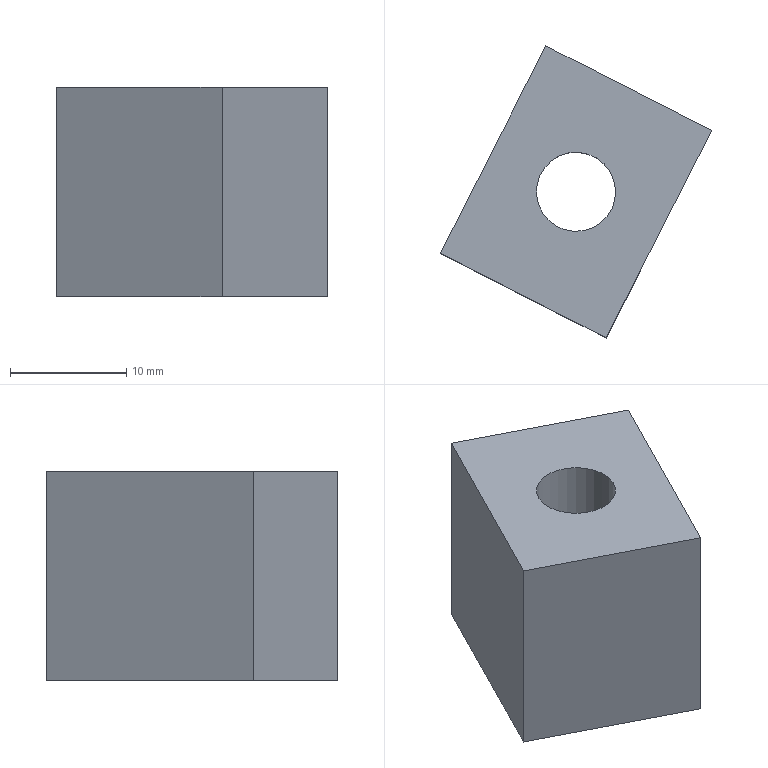Part | STEP file | gslz 2016.10.28-13_id1826_x_t | 1 solid | 9 faces | box 23.336 x 25.084 x 18 mm | volume 4338 mm3 | plane 7 | cylinder 2 | commonest cylinder face diameters 6.8 x1 12 x1
STEP:
#1=CARTESIAN_POINT('',(0.,0.,0.));
#2=DIRECTION('',(0.,0.,1.));
#3=DIRECTION('',(1.,0.,0.));
#4=AXIS2_PLACEMENT_3D('',#1,#2,#3);
#5=CARTESIAN_POINT('',(1096.964,-63.507,-70.5));
#6=VERTEX_POINT('',#5);
#7=CARTESIAN_POINT('',(1106.043,-45.687,-70.5));
#8=VERTEX_POINT('',#7);
#9=CARTESIAN_POINT('',(1103.234,-51.201,-70.5));
#10=DIRECTION('',(0.454,0.891,0.));
#11=VECTOR('',#10,1.);
#12=LINE('',#9,#11);
#13=CARTESIAN_POINT('',(1096.056,-65.289,-97.82));
#14=DIRECTION('',(-0.891,0.454,0.));
#15=DIRECTION('',(0.454,0.891,0.));
#16=AXIS2_PLACEMENT_3D('',#13,#14,#15);
#17=PLANE('',#16);
#18=CARTESIAN_POINT('',(15.812,-27.32));
#19=DIRECTION('',(1.,0.));
#20=VECTOR('',#19,1.);
#21=LINE('',#18,#20);
#22=(GEOMETRIC_REPRESENTATION_CONTEXT(2)PARAMETRIC_REPRESENTATION_CONTEXT()REPRESENTATION_CONTEXT('',''));
#23=DEFINITIONAL_REPRESENTATION('',(#21),#22);
#24=PCURVE('',#17,#23);
#25=CARTESIAN_POINT('',(1099.199,-49.145,-70.5));
#26=DIRECTION('',(0.,0.,1.));
#27=DIRECTION('',(-0.309,0.9511,0.));
#28=AXIS2_PLACEMENT_3D('',#25,#26,#27);
#29=PLANE('',#28);
#30=CARTESIAN_POINT('',(-3.202,-3.202));
#31=DIRECTION('',(0.7071,-0.7071));
#32=VECTOR('',#31,1.);
#33=LINE('',#30,#32);
#34=(GEOMETRIC_REPRESENTATION_CONTEXT(2)PARAMETRIC_REPRESENTATION_CONTEXT()REPRESENTATION_CONTEXT('',''));
#35=DEFINITIONAL_REPRESENTATION('',(#33),#34);
#36=PCURVE('',#29,#35);
#37=SURFACE_CURVE('',#12,(#24,#36),.PCURVE_S1.);
#38=EDGE_CURVE('',#6,#8,#37,.T.);
#39=ORIENTED_EDGE('',*,*,#38,.T.);
#40=CARTESIAN_POINT('',(1106.043,-45.687,-88.5));
#41=VERTEX_POINT('',#40);
#42=CARTESIAN_POINT('',(1106.043,-45.687,-97.82));
#43=DIRECTION('',(0.,0.,1.));
#44=VECTOR('',#43,1.);
#45=LINE('',#42,#44);
#46=CARTESIAN_POINT('',(22.,0.));
#47=DIRECTION('',(0.,-1.));
#48=VECTOR('',#47,1.);
#49=LINE('',#46,#48);
#50=(GEOMETRIC_REPRESENTATION_CONTEXT(2)PARAMETRIC_REPRESENTATION_CONTEXT()REPRESENTATION_CONTEXT('',''));
#51=DEFINITIONAL_REPRESENTATION('',(#49),#50);
#52=PCURVE('',#17,#51);
#53=CARTESIAN_POINT('',(1102.479,-43.871,-97.82));
#54=DIRECTION('',(0.454,0.891,0.));
#55=DIRECTION('',(0.891,-0.454,0.));
#56=AXIS2_PLACEMENT_3D('',#53,#54,#55);
#57=PLANE('',#56);
#58=CARTESIAN_POINT('',(4.,0.));
#59=DIRECTION('',(0.,-1.));
#60=VECTOR('',#59,1.);
#61=LINE('',#58,#60);
#62=(GEOMETRIC_REPRESENTATION_CONTEXT(2)PARAMETRIC_REPRESENTATION_CONTEXT()REPRESENTATION_CONTEXT('',''));
#63=DEFINITIONAL_REPRESENTATION('',(#61),#62);
#64=PCURVE('',#57,#63);
#65=SURFACE_CURVE('',#45,(#52,#64),.PCURVE_S1.);
#66=EDGE_CURVE('',#41,#8,#65,.T.);
#67=ORIENTED_EDGE('',*,*,#66,.F.);
#68=CARTESIAN_POINT('',(1096.964,-63.507,-88.5));
#69=VERTEX_POINT('',#68);
#70=CARTESIAN_POINT('',(1103.234,-51.201,-88.5));
#71=DIRECTION('',(0.454,0.891,0.));
#72=VECTOR('',#71,1.);
#73=LINE('',#70,#72);
#74=CARTESIAN_POINT('',(15.812,-9.32));
#75=DIRECTION('',(1.,0.));
#76=VECTOR('',#75,1.);
#77=LINE('',#74,#76);
#78=(GEOMETRIC_REPRESENTATION_CONTEXT(2)PARAMETRIC_REPRESENTATION_CONTEXT()REPRESENTATION_CONTEXT('',''));
#79=DEFINITIONAL_REPRESENTATION('',(#77),#78);
#80=PCURVE('',#17,#79);
#81=CARTESIAN_POINT('',(1099.199,-49.145,-88.5));
#82=DIRECTION('',(0.,0.,1.));
#83=DIRECTION('',(-0.309,0.9511,0.));
#84=AXIS2_PLACEMENT_3D('',#81,#82,#83);
#85=PLANE('',#84);
#86=CARTESIAN_POINT('',(-3.202,-3.202));
#87=DIRECTION('',(0.7071,-0.7071));
#88=VECTOR('',#87,1.);
#89=LINE('',#86,#88);
#90=(GEOMETRIC_REPRESENTATION_CONTEXT(2)PARAMETRIC_REPRESENTATION_CONTEXT()REPRESENTATION_CONTEXT('',''));
#91=DEFINITIONAL_REPRESENTATION('',(#89),#90);
#92=PCURVE('',#85,#91);
#93=SURFACE_CURVE('',#73,(#80,#92),.PCURVE_S1.);
#94=EDGE_CURVE('',#69,#41,#93,.T.);
#95=ORIENTED_EDGE('',*,*,#94,.F.);
#96=CARTESIAN_POINT('',(1096.964,-63.507,-97.82));
#97=DIRECTION('',(0.,0.,1.));
#98=VECTOR('',#97,1.);
#99=LINE('',#96,#98);
#100=CARTESIAN_POINT('',(2.,0.));
#101=DIRECTION('',(0.,-1.));
#102=VECTOR('',#101,1.);
#103=LINE('',#100,#102);
#104=(GEOMETRIC_REPRESENTATION_CONTEXT(2)PARAMETRIC_REPRESENTATION_CONTEXT()REPRESENTATION_CONTEXT('',''));
#105=DEFINITIONAL_REPRESENTATION('',(#103),#104);
#106=PCURVE('',#17,#105);
#107=CARTESIAN_POINT('',(1114.784,-72.587,-97.82));
#108=DIRECTION('',(-0.454,-0.891,0.));
#109=DIRECTION('',(-0.891,0.454,0.));
#110=AXIS2_PLACEMENT_3D('',#107,#108,#109);
#111=PLANE('',#110);
#112=CARTESIAN_POINT('',(20.,0.));
#113=DIRECTION('',(0.,-1.));
#114=VECTOR('',#113,1.);
#115=LINE('',#112,#114);
#116=(GEOMETRIC_REPRESENTATION_CONTEXT(2)PARAMETRIC_REPRESENTATION_CONTEXT()REPRESENTATION_CONTEXT('',''));
#117=DEFINITIONAL_REPRESENTATION('',(#115),#116);
#118=PCURVE('',#111,#117);
#119=SURFACE_CURVE('',#99,(#106,#118),.PCURVE_S1.);
#120=EDGE_CURVE('',#69,#6,#119,.T.);
#121=ORIENTED_EDGE('',*,*,#120,.T.);
#122=EDGE_LOOP('',(#39,#67,#95,#121));
#123=FACE_BOUND('',#122,.T.);
#124=ADVANCED_FACE('',(#123),#17,.T.);
#125=CARTESIAN_POINT('',(1120.299,-52.951,-70.5));
#126=VERTEX_POINT('',#125);
#127=CARTESIAN_POINT('',(1102.008,-43.631,-70.5));
#128=DIRECTION('',(0.891,-0.454,0.));
#129=VECTOR('',#128,1.);
#130=LINE('',#127,#129);
#131=CARTESIAN_POINT('',(-0.5289,-27.32));
#132=DIRECTION('',(1.,0.));
#133=VECTOR('',#132,1.);
#134=LINE('',#131,#133);
#135=(GEOMETRIC_REPRESENTATION_CONTEXT(2)PARAMETRIC_REPRESENTATION_CONTEXT()REPRESENTATION_CONTEXT('',''));
#136=DEFINITIONAL_REPRESENTATION('',(#134),#135);
#137=PCURVE('',#57,#136);
#138=CARTESIAN_POINT('',(4.376,-4.376));
#139=DIRECTION('',(-0.7071,-0.7071));
#140=VECTOR('',#139,1.);
#141=LINE('',#138,#140);
#142=(GEOMETRIC_REPRESENTATION_CONTEXT(2)PARAMETRIC_REPRESENTATION_CONTEXT()REPRESENTATION_CONTEXT('',''));
#143=DEFINITIONAL_REPRESENTATION('',(#141),#142);
#144=PCURVE('',#29,#143);
#145=SURFACE_CURVE('',#130,(#137,#144),.PCURVE_S1.);
#146=EDGE_CURVE('',#8,#126,#145,.T.);
#147=ORIENTED_EDGE('',*,*,#146,.T.);
#148=CARTESIAN_POINT('',(1120.299,-52.951,-88.5));
#149=VERTEX_POINT('',#148);
#150=CARTESIAN_POINT('',(1120.299,-52.951,-97.82));
#151=DIRECTION('',(0.,0.,1.));
#152=VECTOR('',#151,1.);
#153=LINE('',#150,#152);
#154=CARTESIAN_POINT('',(20.,0.));
#155=DIRECTION('',(0.,-1.));
#156=VECTOR('',#155,1.);
#157=LINE('',#154,#156);
#158=(GEOMETRIC_REPRESENTATION_CONTEXT(2)PARAMETRIC_REPRESENTATION_CONTEXT()REPRESENTATION_CONTEXT('',''));
#159=DEFINITIONAL_REPRESENTATION('',(#157),#158);
#160=PCURVE('',#57,#159);
#161=CARTESIAN_POINT('',(1121.207,-51.169,-97.82));
#162=DIRECTION('',(0.891,-0.454,0.));
#163=DIRECTION('',(-0.454,-0.891,0.));
#164=AXIS2_PLACEMENT_3D('',#161,#162,#163);
#165=PLANE('',#164);
#166=CARTESIAN_POINT('',(2.,0.));
#167=DIRECTION('',(0.,-1.));
#168=VECTOR('',#167,1.);
#169=LINE('',#166,#168);
#170=(GEOMETRIC_REPRESENTATION_CONTEXT(2)PARAMETRIC_REPRESENTATION_CONTEXT()REPRESENTATION_CONTEXT('',''));
#171=DEFINITIONAL_REPRESENTATION('',(#169),#170);
#172=PCURVE('',#165,#171);
#173=SURFACE_CURVE('',#153,(#160,#172),.PCURVE_S1.);
#174=EDGE_CURVE('',#149,#126,#173,.T.);
#175=ORIENTED_EDGE('',*,*,#174,.F.);
#176=CARTESIAN_POINT('',(1102.008,-43.631,-88.5));
#177=DIRECTION('',(0.891,-0.454,0.));
#178=VECTOR('',#177,1.);
#179=LINE('',#176,#178);
#180=CARTESIAN_POINT('',(-0.5289,-9.32));
#181=DIRECTION('',(1.,0.));
#182=VECTOR('',#181,1.);
#183=LINE('',#180,#182);
#184=(GEOMETRIC_REPRESENTATION_CONTEXT(2)PARAMETRIC_REPRESENTATION_CONTEXT()REPRESENTATION_CONTEXT('',''));
#185=DEFINITIONAL_REPRESENTATION('',(#183),#184);
#186=PCURVE('',#57,#185);
#187=CARTESIAN_POINT('',(4.376,-4.376));
#188=DIRECTION('',(-0.7071,-0.7071));
#189=VECTOR('',#188,1.);
#190=LINE('',#187,#189);
#191=(GEOMETRIC_REPRESENTATION_CONTEXT(2)PARAMETRIC_REPRESENTATION_CONTEXT()REPRESENTATION_CONTEXT('',''));
#192=DEFINITIONAL_REPRESENTATION('',(#190),#191);
#193=PCURVE('',#85,#192);
#194=SURFACE_CURVE('',#179,(#186,#193),.PCURVE_S1.);
#195=EDGE_CURVE('',#41,#149,#194,.T.);
#196=ORIENTED_EDGE('',*,*,#195,.F.);
#197=ORIENTED_EDGE('',*,*,#66,.T.);
#198=EDGE_LOOP('',(#147,#175,#196,#197));
#199=FACE_BOUND('',#198,.T.);
#200=ADVANCED_FACE('',(#199),#57,.T.);
#201=CARTESIAN_POINT('',(1111.22,-70.771,-70.5));
#202=VERTEX_POINT('',#201);
#203=CARTESIAN_POINT('',(1117.49,-58.465,-70.5));
#204=DIRECTION('',(-0.454,-0.891,0.));
#205=VECTOR('',#204,1.);
#206=LINE('',#203,#205);
#207=CARTESIAN_POINT('',(8.188,-27.32));
#208=DIRECTION('',(1.,0.));
#209=VECTOR('',#208,1.);
#210=LINE('',#207,#209);
#211=(GEOMETRIC_REPRESENTATION_CONTEXT(2)PARAMETRIC_REPRESENTATION_CONTEXT()REPRESENTATION_CONTEXT('',''));
#212=DEFINITIONAL_REPRESENTATION('',(#210),#211);
#213=PCURVE('',#165,#212);
#214=CARTESIAN_POINT('',(-14.516,-14.516));
#215=DIRECTION('',(-0.7071,0.7071));
#216=VECTOR('',#215,1.);
#217=LINE('',#214,#216);
#218=(GEOMETRIC_REPRESENTATION_CONTEXT(2)PARAMETRIC_REPRESENTATION_CONTEXT()REPRESENTATION_CONTEXT('',''));
#219=DEFINITIONAL_REPRESENTATION('',(#217),#218);
#220=PCURVE('',#29,#219);
#221=SURFACE_CURVE('',#206,(#213,#220),.PCURVE_S1.);
#222=EDGE_CURVE('',#126,#202,#221,.T.);
#223=ORIENTED_EDGE('',*,*,#222,.T.);
#224=CARTESIAN_POINT('',(1111.22,-70.771,-88.5));
#225=VERTEX_POINT('',#224);
#226=CARTESIAN_POINT('',(1111.22,-70.771,-97.82));
#227=DIRECTION('',(0.,0.,1.));
#228=VECTOR('',#227,1.);
#229=LINE('',#226,#228);
#230=CARTESIAN_POINT('',(22.,0.));
#231=DIRECTION('',(0.,-1.));
#232=VECTOR('',#231,1.);
#233=LINE('',#230,#232);
#234=(GEOMETRIC_REPRESENTATION_CONTEXT(2)PARAMETRIC_REPRESENTATION_CONTEXT()REPRESENTATION_CONTEXT('',''));
#235=DEFINITIONAL_REPRESENTATION('',(#233),#234);
#236=PCURVE('',#165,#235);
#237=CARTESIAN_POINT('',(4.,0.));
#238=DIRECTION('',(0.,-1.));
#239=VECTOR('',#238,1.);
#240=LINE('',#237,#239);
#241=(GEOMETRIC_REPRESENTATION_CONTEXT(2)PARAMETRIC_REPRESENTATION_CONTEXT()REPRESENTATION_CONTEXT('',''));
#242=DEFINITIONAL_REPRESENTATION('',(#240),#241);
#243=PCURVE('',#111,#242);
#244=SURFACE_CURVE('',#229,(#236,#243),.PCURVE_S1.);
#245=EDGE_CURVE('',#225,#202,#244,.T.);
#246=ORIENTED_EDGE('',*,*,#245,.F.);
#247=CARTESIAN_POINT('',(1117.49,-58.465,-88.5));
#248=DIRECTION('',(-0.454,-0.891,0.));
#249=VECTOR('',#248,1.);
#250=LINE('',#247,#249);
#251=CARTESIAN_POINT('',(8.188,-9.32));
#252=DIRECTION('',(1.,0.));
#253=VECTOR('',#252,1.);
#254=LINE('',#251,#253);
#255=(GEOMETRIC_REPRESENTATION_CONTEXT(2)PARAMETRIC_REPRESENTATION_CONTEXT()REPRESENTATION_CONTEXT('',''));
#256=DEFINITIONAL_REPRESENTATION('',(#254),#255);
#257=PCURVE('',#165,#256);
#258=CARTESIAN_POINT('',(-14.516,-14.516));
#259=DIRECTION('',(-0.7071,0.7071));
#260=VECTOR('',#259,1.);
#261=LINE('',#258,#260);
#262=(GEOMETRIC_REPRESENTATION_CONTEXT(2)PARAMETRIC_REPRESENTATION_CONTEXT()REPRESENTATION_CONTEXT('',''));
#263=DEFINITIONAL_REPRESENTATION('',(#261),#262);
#264=PCURVE('',#85,#263);
#265=SURFACE_CURVE('',#250,(#257,#264),.PCURVE_S1.);
#266=EDGE_CURVE('',#149,#225,#265,.T.);
#267=ORIENTED_EDGE('',*,*,#266,.F.);
#268=ORIENTED_EDGE('',*,*,#174,.T.);
#269=EDGE_LOOP('',(#223,#246,#267,#268));
#270=FACE_BOUND('',#269,.T.);
#271=ADVANCED_FACE('',(#270),#165,.T.);
#272=CARTESIAN_POINT('',(1092.928,-61.451,-70.5));
#273=DIRECTION('',(-0.891,0.454,0.));
#274=VECTOR('',#273,1.);
#275=LINE('',#272,#274);
#276=CARTESIAN_POINT('',(24.529,-27.32));
#277=DIRECTION('',(1.,0.));
#278=VECTOR('',#277,1.);
#279=LINE('',#276,#278);
#280=(GEOMETRIC_REPRESENTATION_CONTEXT(2)PARAMETRIC_REPRESENTATION_CONTEXT()REPRESENTATION_CONTEXT('',''));
#281=DEFINITIONAL_REPRESENTATION('',(#279),#280);
#282=PCURVE('',#111,#281);
#283=CARTESIAN_POINT('',(-9.766,9.766));
#284=DIRECTION('',(0.7071,0.7071));
#285=VECTOR('',#284,1.);
#286=LINE('',#283,#285);
#287=(GEOMETRIC_REPRESENTATION_CONTEXT(2)PARAMETRIC_REPRESENTATION_CONTEXT()REPRESENTATION_CONTEXT('',''));
#288=DEFINITIONAL_REPRESENTATION('',(#286),#287);
#289=PCURVE('',#29,#288);
#290=SURFACE_CURVE('',#275,(#282,#289),.PCURVE_S1.);
#291=EDGE_CURVE('',#202,#6,#290,.T.);
#292=ORIENTED_EDGE('',*,*,#291,.T.);
#293=ORIENTED_EDGE('',*,*,#120,.F.);
#294=CARTESIAN_POINT('',(1092.928,-61.451,-88.5));
#295=DIRECTION('',(-0.891,0.454,0.));
#296=VECTOR('',#295,1.);
#297=LINE('',#294,#296);
#298=CARTESIAN_POINT('',(24.529,-9.32));
#299=DIRECTION('',(1.,0.));
#300=VECTOR('',#299,1.);
#301=LINE('',#298,#300);
#302=(GEOMETRIC_REPRESENTATION_CONTEXT(2)PARAMETRIC_REPRESENTATION_CONTEXT()REPRESENTATION_CONTEXT('',''));
#303=DEFINITIONAL_REPRESENTATION('',(#301),#302);
#304=PCURVE('',#111,#303);
#305=CARTESIAN_POINT('',(-9.766,9.766));
#306=DIRECTION('',(0.7071,0.7071));
#307=VECTOR('',#306,1.);
#308=LINE('',#305,#307);
#309=(GEOMETRIC_REPRESENTATION_CONTEXT(2)PARAMETRIC_REPRESENTATION_CONTEXT()REPRESENTATION_CONTEXT('',''));
#310=DEFINITIONAL_REPRESENTATION('',(#308),#309);
#311=PCURVE('',#85,#310);
#312=SURFACE_CURVE('',#297,(#304,#311),.PCURVE_S1.);
#313=EDGE_CURVE('',#225,#69,#312,.T.);
#314=ORIENTED_EDGE('',*,*,#313,.F.);
#315=ORIENTED_EDGE('',*,*,#245,.T.);
#316=EDGE_LOOP('',(#292,#293,#314,#315));
#317=FACE_BOUND('',#316,.T.);
#318=ADVANCED_FACE('',(#317),#111,.T.);
#319=CARTESIAN_POINT('',(1112.325,-62.957,-88.5));
#320=VERTEX_POINT('',#319);
#321=CARTESIAN_POINT('',(1108.631,-58.229,-88.5));
#322=DIRECTION('',(0.,0.,-1.));
#323=DIRECTION('',(0.6157,-0.788,0.));
#324=AXIS2_PLACEMENT_3D('',#321,#322,#323);
#325=CIRCLE('',#324,6.);
#326=CARTESIAN_POINT('',(-17.193,-8.216));
#327=CARTESIAN_POINT('',(-20.747,1.549));
#328=CARTESIAN_POINT('',(-10.513,-0.2553));
#329=CARTESIAN_POINT('',(-0.2782,-2.06));
#330=CARTESIAN_POINT('',(-6.958,-10.021));
#331=CARTESIAN_POINT('',(-13.638,-17.982));
#332=CARTESIAN_POINT('',(-17.193,-8.216));
#333=(BOUNDED_CURVE()B_SPLINE_CURVE(2,(#326,#327,#328,#329,#330,#331,#332),.UNSPECIFIED.,.T.,.F.)B_SPLINE_CURVE_WITH_KNOTS((1,2,2,2,2,1),(-2.094,0.,2.094,4.189,6.283,8.378),.UNSPECIFIED.)CURVE()GEOMETRIC_REPRESENTATION_ITEM()RATIONAL_B_SPLINE_CURVE((1.,0.5,1.,0.5,1.,0.5,1.))REPRESENTATION_ITEM(''));
#334=(GEOMETRIC_REPRESENTATION_CONTEXT(2)PARAMETRIC_REPRESENTATION_CONTEXT()REPRESENTATION_CONTEXT('',''));
#335=DEFINITIONAL_REPRESENTATION('',(#333),#334);
#336=PCURVE('',#85,#335);
#337=CARTESIAN_POINT('',(1108.631,-58.229,-97.82));
#338=DIRECTION('',(0.,0.,1.));
#339=DIRECTION('',(0.9064,-0.4223,0.));
#340=AXIS2_PLACEMENT_3D('',#337,#338,#339);
#341=CYLINDRICAL_SURFACE('',#340,6.);
#342=CARTESIAN_POINT('',(12.095,9.32));
#343=DIRECTION('',(-1.,0.));
#344=VECTOR('',#343,1.);
#345=LINE('',#342,#344);
#346=(GEOMETRIC_REPRESENTATION_CONTEXT(2)PARAMETRIC_REPRESENTATION_CONTEXT()REPRESENTATION_CONTEXT('',''));
#347=DEFINITIONAL_REPRESENTATION('',(#345),#346);
#348=PCURVE('',#341,#347);
#349=SURFACE_CURVE('',#325,(#336,#348),.PCURVE_S1.);
#350=EDGE_CURVE('',#320,#320,#349,.T.);
#351=ORIENTED_EDGE('',*,*,#350,.F.);
#352=EDGE_LOOP('',(#351));
#353=FACE_BOUND('',#352,.T.);
#354=ORIENTED_EDGE('',*,*,#94,.T.);
#355=ORIENTED_EDGE('',*,*,#195,.T.);
#356=ORIENTED_EDGE('',*,*,#266,.T.);
#357=ORIENTED_EDGE('',*,*,#313,.T.);
#358=EDGE_LOOP('',(#354,#355,#356,#357));
#359=FACE_BOUND('',#358,.T.);
#360=ADVANCED_FACE('',(#353,#359),#85,.F.);
#361=CARTESIAN_POINT('',(1110.725,-60.909,-70.5));
#362=VERTEX_POINT('',#361);
#363=CARTESIAN_POINT('',(1108.631,-58.229,-70.5));
#364=DIRECTION('',(0.,0.,-1.));
#365=DIRECTION('',(0.6157,-0.788,0.));
#366=AXIS2_PLACEMENT_3D('',#363,#364,#365);
#367=CIRCLE('',#366,3.4);
#368=CARTESIAN_POINT('',(-14.749,-7.327));
#369=CARTESIAN_POINT('',(-16.764,-1.793));
#370=CARTESIAN_POINT('',(-10.964,-2.816));
#371=CARTESIAN_POINT('',(-5.165,-3.838));
#372=CARTESIAN_POINT('',(-8.95,-8.35));
#373=CARTESIAN_POINT('',(-12.735,-12.861));
#374=CARTESIAN_POINT('',(-14.749,-7.327));
#375=(BOUNDED_CURVE()B_SPLINE_CURVE(2,(#368,#369,#370,#371,#372,#373,#374),.UNSPECIFIED.,.T.,.F.)B_SPLINE_CURVE_WITH_KNOTS((1,2,2,2,2,1),(-2.094,0.,2.094,4.189,6.283,8.378),.UNSPECIFIED.)CURVE()GEOMETRIC_REPRESENTATION_ITEM()RATIONAL_B_SPLINE_CURVE((1.,0.5,1.,0.5,1.,0.5,1.))REPRESENTATION_ITEM(''));
#376=(GEOMETRIC_REPRESENTATION_CONTEXT(2)PARAMETRIC_REPRESENTATION_CONTEXT()REPRESENTATION_CONTEXT('',''));
#377=DEFINITIONAL_REPRESENTATION('',(#375),#376);
#378=PCURVE('',#29,#377);
#379=CARTESIAN_POINT('',(1108.631,-58.229,-47.82));
#380=DIRECTION('',(0.,0.,1.));
#381=DIRECTION('',(0.9064,-0.4223,0.));
#382=AXIS2_PLACEMENT_3D('',#379,#380,#381);
#383=CYLINDRICAL_SURFACE('',#382,3.4);
#384=CARTESIAN_POINT('',(12.095,-22.68));
#385=DIRECTION('',(-1.,0.));
#386=VECTOR('',#385,1.);
#387=LINE('',#384,#386);
#388=(GEOMETRIC_REPRESENTATION_CONTEXT(2)PARAMETRIC_REPRESENTATION_CONTEXT()REPRESENTATION_CONTEXT('',''));
#389=DEFINITIONAL_REPRESENTATION('',(#387),#388);
#390=PCURVE('',#383,#389);
#391=SURFACE_CURVE('',#367,(#378,#390),.PCURVE_S1.);
#392=EDGE_CURVE('',#362,#362,#391,.T.);
#393=ORIENTED_EDGE('',*,*,#392,.T.);
#394=EDGE_LOOP('',(#393));
#395=FACE_BOUND('',#394,.T.);
#396=ORIENTED_EDGE('',*,*,#38,.F.);
#397=ORIENTED_EDGE('',*,*,#291,.F.);
#398=ORIENTED_EDGE('',*,*,#222,.F.);
#399=ORIENTED_EDGE('',*,*,#146,.F.);
#400=EDGE_LOOP('',(#396,#397,#398,#399));
#401=FACE_BOUND('',#400,.T.);
#402=ADVANCED_FACE('',(#395,#401),#29,.T.);
#403=ORIENTED_EDGE('',*,*,#392,.T.);
#404=CARTESIAN_POINT('',(1110.725,-60.909,-78.5));
#405=VERTEX_POINT('',#404);
#406=CARTESIAN_POINT('',(1110.725,-60.909,-78.5));
#407=CARTESIAN_POINT('',(1110.725,-60.909,-70.5));
#408=B_SPLINE_CURVE_WITH_KNOTS('',1,(#406,#407),.UNSPECIFIED.,.F.,.F.,(2,2),(-30.68,-22.68),.PIECEWISE_BEZIER_KNOTS.);
#409=CARTESIAN_POINT('',(5.812,0.));
#410=DIRECTION('',(0.,1.));
#411=VECTOR('',#410,1.);
#412=LINE('',#409,#411);
#413=(GEOMETRIC_REPRESENTATION_CONTEXT(2)PARAMETRIC_REPRESENTATION_CONTEXT()REPRESENTATION_CONTEXT('',''));
#414=DEFINITIONAL_REPRESENTATION('',(#412),#413);
#415=PCURVE('',#383,#414);
#416=CARTESIAN_POINT('',(12.095,0.));
#417=DIRECTION('',(0.,1.));
#418=VECTOR('',#417,1.);
#419=LINE('',#416,#418);
#420=(GEOMETRIC_REPRESENTATION_CONTEXT(2)PARAMETRIC_REPRESENTATION_CONTEXT()REPRESENTATION_CONTEXT('',''));
#421=DEFINITIONAL_REPRESENTATION('',(#419),#420);
#422=PCURVE('',#383,#421);
#423=SEAM_CURVE('',#408,(#415,#422),.PCURVE_S1.);
#424=EDGE_CURVE('',#405,#362,#423,.T.);
#425=ORIENTED_EDGE('',*,*,#424,.F.);
#426=CARTESIAN_POINT('',(1108.631,-58.229,-78.5));
#427=DIRECTION('',(0.,0.,-1.));
#428=DIRECTION('',(0.6157,-0.788,0.));
#429=AXIS2_PLACEMENT_3D('',#426,#427,#428);
#430=CIRCLE('',#429,3.4);
#431=CARTESIAN_POINT('',(12.095,-30.68));
#432=DIRECTION('',(-1.,0.));
#433=VECTOR('',#432,1.);
#434=LINE('',#431,#433);
#435=(GEOMETRIC_REPRESENTATION_CONTEXT(2)PARAMETRIC_REPRESENTATION_CONTEXT()REPRESENTATION_CONTEXT('',''));
#436=DEFINITIONAL_REPRESENTATION('',(#434),#435);
#437=PCURVE('',#383,#436);
#438=CARTESIAN_POINT('',(1099.199,-49.145,-78.5));
#439=DIRECTION('',(0.,0.,1.));
#440=DIRECTION('',(-0.309,0.9511,0.));
#441=AXIS2_PLACEMENT_3D('',#438,#439,#440);
#442=PLANE('',#441);
#443=CARTESIAN_POINT('',(-14.749,-7.327));
#444=CARTESIAN_POINT('',(-16.764,-1.793));
#445=CARTESIAN_POINT('',(-10.964,-2.816));
#446=CARTESIAN_POINT('',(-5.165,-3.838));
#447=CARTESIAN_POINT('',(-8.95,-8.35));
#448=CARTESIAN_POINT('',(-12.735,-12.861));
#449=CARTESIAN_POINT('',(-14.749,-7.327));
#450=(BOUNDED_CURVE()B_SPLINE_CURVE(2,(#443,#444,#445,#446,#447,#448,#449),.UNSPECIFIED.,.T.,.F.)B_SPLINE_CURVE_WITH_KNOTS((1,2,2,2,2,1),(-2.094,0.,2.094,4.189,6.283,8.378),.UNSPECIFIED.)CURVE()GEOMETRIC_REPRESENTATION_ITEM()RATIONAL_B_SPLINE_CURVE((1.,0.5,1.,0.5,1.,0.5,1.))REPRESENTATION_ITEM(''));
#451=(GEOMETRIC_REPRESENTATION_CONTEXT(2)PARAMETRIC_REPRESENTATION_CONTEXT()REPRESENTATION_CONTEXT('',''));
#452=DEFINITIONAL_REPRESENTATION('',(#450),#451);
#453=PCURVE('',#442,#452);
#454=SURFACE_CURVE('',#430,(#437,#453),.PCURVE_S1.);
#455=EDGE_CURVE('',#405,#405,#454,.T.);
#456=ORIENTED_EDGE('',*,*,#455,.F.);
#457=ORIENTED_EDGE('',*,*,#424,.T.);
#458=EDGE_LOOP('',(#403,#425,#456,#457));
#459=FACE_BOUND('',#458,.F.);
#460=ADVANCED_FACE('',(#459),#383,.F.);
#461=ORIENTED_EDGE('',*,*,#455,.F.);
#462=EDGE_LOOP('',(#461));
#463=FACE_BOUND('',#462,.T.);
#464=CARTESIAN_POINT('',(1112.325,-62.957,-78.5));
#465=VERTEX_POINT('',#464);
#466=CARTESIAN_POINT('',(1108.631,-58.229,-78.5));
#467=DIRECTION('',(0.,0.,-1.));
#468=DIRECTION('',(0.6157,-0.788,0.));
#469=AXIS2_PLACEMENT_3D('',#466,#467,#468);
#470=CIRCLE('',#469,6.);
#471=CARTESIAN_POINT('',(-17.193,-8.216));
#472=CARTESIAN_POINT('',(-20.747,1.549));
#473=CARTESIAN_POINT('',(-10.513,-0.2553));
#474=CARTESIAN_POINT('',(-0.2782,-2.06));
#475=CARTESIAN_POINT('',(-6.958,-10.021));
#476=CARTESIAN_POINT('',(-13.638,-17.982));
#477=CARTESIAN_POINT('',(-17.193,-8.216));
#478=(BOUNDED_CURVE()B_SPLINE_CURVE(2,(#471,#472,#473,#474,#475,#476,#477),.UNSPECIFIED.,.T.,.F.)B_SPLINE_CURVE_WITH_KNOTS((1,2,2,2,2,1),(-2.094,0.,2.094,4.189,6.283,8.378),.UNSPECIFIED.)CURVE()GEOMETRIC_REPRESENTATION_ITEM()RATIONAL_B_SPLINE_CURVE((1.,0.5,1.,0.5,1.,0.5,1.))REPRESENTATION_ITEM(''));
#479=(GEOMETRIC_REPRESENTATION_CONTEXT(2)PARAMETRIC_REPRESENTATION_CONTEXT()REPRESENTATION_CONTEXT('',''));
#480=DEFINITIONAL_REPRESENTATION('',(#478),#479);
#481=PCURVE('',#442,#480);
#482=CARTESIAN_POINT('',(12.095,19.32));
#483=DIRECTION('',(-1.,0.));
#484=VECTOR('',#483,1.);
#485=LINE('',#482,#484);
#486=(GEOMETRIC_REPRESENTATION_CONTEXT(2)PARAMETRIC_REPRESENTATION_CONTEXT()REPRESENTATION_CONTEXT('',''));
#487=DEFINITIONAL_REPRESENTATION('',(#485),#486);
#488=PCURVE('',#341,#487);
#489=SURFACE_CURVE('',#470,(#481,#488),.PCURVE_S1.);
#490=EDGE_CURVE('',#465,#465,#489,.T.);
#491=ORIENTED_EDGE('',*,*,#490,.T.);
#492=EDGE_LOOP('',(#491));
#493=FACE_BOUND('',#492,.T.);
#494=ADVANCED_FACE('',(#463,#493),#442,.F.);
#495=ORIENTED_EDGE('',*,*,#490,.T.);
#496=CARTESIAN_POINT('',(1112.325,-62.957,-88.5));
#497=CARTESIAN_POINT('',(1112.325,-62.957,-78.5));
#498=B_SPLINE_CURVE_WITH_KNOTS('',1,(#496,#497),.UNSPECIFIED.,.F.,.F.,(2,2),(9.32,19.32),.PIECEWISE_BEZIER_KNOTS.);
#499=CARTESIAN_POINT('',(5.812,0.));
#500=DIRECTION('',(0.,1.));
#501=VECTOR('',#500,1.);
#502=LINE('',#499,#501);
#503=(GEOMETRIC_REPRESENTATION_CONTEXT(2)PARAMETRIC_REPRESENTATION_CONTEXT()REPRESENTATION_CONTEXT('',''));
#504=DEFINITIONAL_REPRESENTATION('',(#502),#503);
#505=PCURVE('',#341,#504);
#506=CARTESIAN_POINT('',(12.095,0.));
#507=DIRECTION('',(0.,1.));
#508=VECTOR('',#507,1.);
#509=LINE('',#506,#508);
#510=(GEOMETRIC_REPRESENTATION_CONTEXT(2)PARAMETRIC_REPRESENTATION_CONTEXT()REPRESENTATION_CONTEXT('',''));
#511=DEFINITIONAL_REPRESENTATION('',(#509),#510);
#512=PCURVE('',#341,#511);
#513=SEAM_CURVE('',#498,(#505,#512),.PCURVE_S1.);
#514=EDGE_CURVE('',#320,#465,#513,.T.);
#515=ORIENTED_EDGE('',*,*,#514,.F.);
#516=ORIENTED_EDGE('',*,*,#350,.F.);
#517=ORIENTED_EDGE('',*,*,#514,.T.);
#518=EDGE_LOOP('',(#495,#515,#516,#517));
#519=FACE_BOUND('',#518,.F.);
#520=ADVANCED_FACE('',(#519),#341,.F.);
#521=CLOSED_SHELL('',(#124,#200,#271,#318,#360,#402,#460,#494,#520));
#522=MANIFOLD_SOLID_BREP('',#521);
#523=(LENGTH_UNIT()NAMED_UNIT(*)SI_UNIT(.MILLI.,.METRE.));
#524=UNCERTAINTY_MEASURE_WITH_UNIT(LENGTH_MEASURE(0.000002),#523,'','');
#525=(NAMED_UNIT(*)PLANE_ANGLE_UNIT()SI_UNIT($,.RADIAN.));
#526=(NAMED_UNIT(*)SI_UNIT($,.STERADIAN.)SOLID_ANGLE_UNIT());
#527=(GEOMETRIC_REPRESENTATION_CONTEXT(3)GLOBAL_UNCERTAINTY_ASSIGNED_CONTEXT((#524))GLOBAL_UNIT_ASSIGNED_CONTEXT((#523,#525,#526))REPRESENTATION_CONTEXT('',''));
#528=ADVANCED_BREP_SHAPE_REPRESENTATION('',(#4,#522),#527);